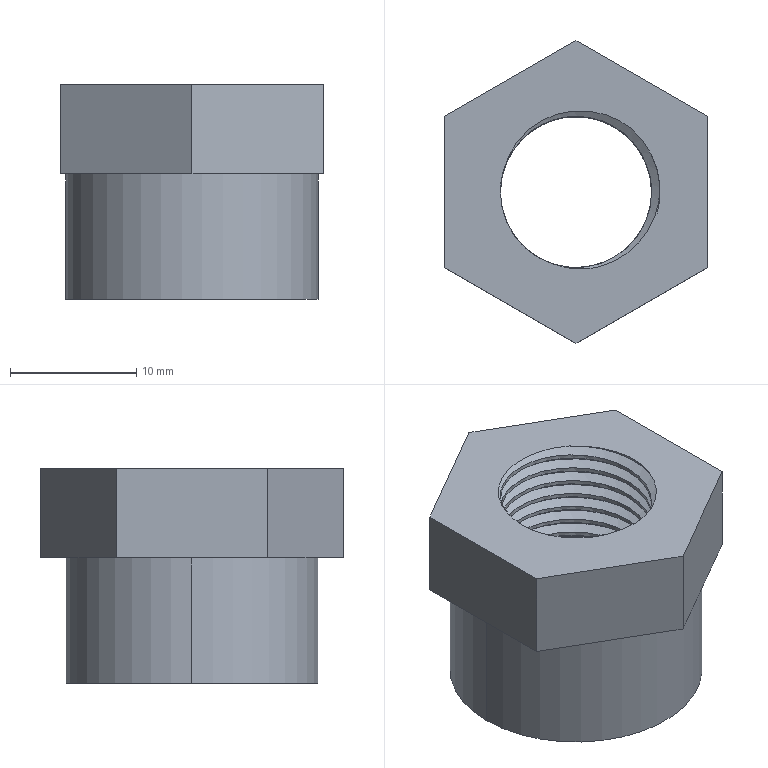Part | SolidWorks | features HoleWzd 1, ICE 1, Revolution 1, SweepThread 1 | 1 solid | 43 faces | box 20.8 x 24.018 x 17 mm | volume 3648 mm3 | cylinder 31 | plane 9 | spline 3 | commonest cylinder face diameters 12 x29 20 x2